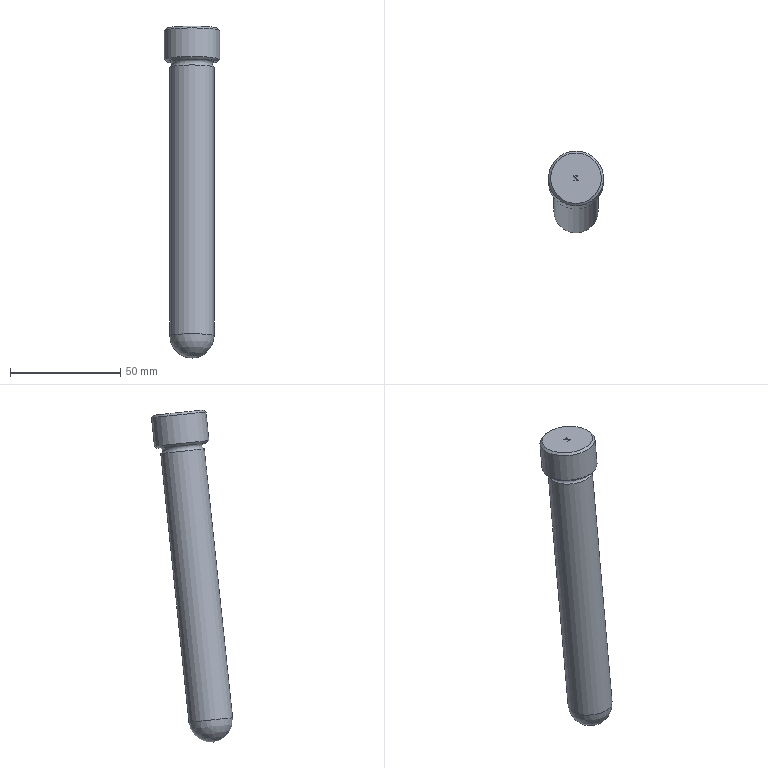Part | STEP file | solid 120 | 1 solid | 19 faces | box 25 x 36.961 x 150.435 mm | volume 48566 mm3 | plane 11 | cylinder 2 | cone 2 | other 2 | sphere 1 | torus 1 | commonest cylinder face diameters 20 x1 25 x1